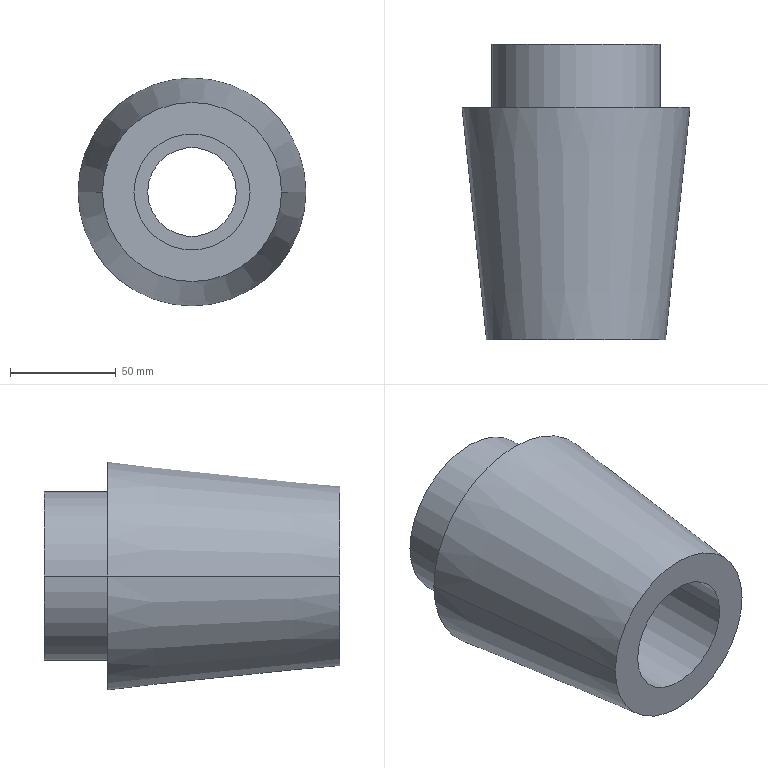Part | STEP file | zhouxin | 1 solid | 18 faces | box 108 x 140 x 108 mm | volume 645082 mm3 | cylinder 10 | plane 6 | cone 2 | commonest cylinder face diameters 4 x4 42 x2 55 x2 80 x2
STEP:
#1=CARTESIAN_POINT('',(2.,-13.333,-32.5));
#2=VERTEX_POINT('',#1);
#3=CARTESIAN_POINT('',(-2.,-13.333,-32.5));
#4=VERTEX_POINT('',#3);
#5=CARTESIAN_POINT('',(0.,-13.333,-32.5));
#6=DIRECTION('',(0.,1.,0.));
#7=DIRECTION('',(-1.,0.,0.));
#8=AXIS2_PLACEMENT_3D('',#5,#6,#7);
#9=CIRCLE('',#8,2.);
#10=EDGE_CURVE('',#2,#4,#9,.T.);
#11=ORIENTED_EDGE('',*,*,#10,.F.);
#12=CARTESIAN_POINT('',(2.,-3.333,-32.5));
#13=VERTEX_POINT('',#12);
#14=CARTESIAN_POINT('',(2.,-13.333,-32.5));
#15=DIRECTION('',(0.,1.,0.));
#16=VECTOR('',#15,1000.);
#17=LINE('',#14,#16);
#18=EDGE_CURVE('',#2,#13,#17,.T.);
#19=ORIENTED_EDGE('',*,*,#18,.T.);
#20=CARTESIAN_POINT('',(-2.,-3.333,-32.5));
#21=VERTEX_POINT('',#20);
#22=CARTESIAN_POINT('',(0.,-3.333,-32.5));
#23=DIRECTION('',(0.,1.,0.));
#24=DIRECTION('',(-1.,0.,0.));
#25=AXIS2_PLACEMENT_3D('',#22,#23,#24);
#26=CIRCLE('',#25,2.);
#27=EDGE_CURVE('',#13,#21,#26,.T.);
#28=ORIENTED_EDGE('',*,*,#27,.T.);
#29=CARTESIAN_POINT('',(-2.,-13.333,-32.5));
#30=DIRECTION('',(0.,1.,0.));
#31=VECTOR('',#30,1000.);
#32=LINE('',#29,#31);
#33=EDGE_CURVE('',#4,#21,#32,.T.);
#34=ORIENTED_EDGE('',*,*,#33,.F.);
#35=EDGE_LOOP('',(#11,#19,#28,#34));
#36=FACE_OUTER_BOUND('',#35,.T.);
#37=CARTESIAN_POINT('',(0.,-13.333,-32.5));
#38=DIRECTION('',(0.,1.,0.));
#39=DIRECTION('',(-1.,0.,0.));
#40=AXIS2_PLACEMENT_3D('',#37,#38,#39);
#41=CYLINDRICAL_SURFACE('',#40,2.);
#42=ADVANCED_FACE('',(#36),#41,.F.);
#43=CARTESIAN_POINT('',(2.,-13.333,32.5));
#44=VERTEX_POINT('',#43);
#45=CARTESIAN_POINT('',(-2.,-13.333,32.5));
#46=VERTEX_POINT('',#45);
#47=CARTESIAN_POINT('',(0.,-13.333,32.5));
#48=DIRECTION('',(0.,1.,0.));
#49=DIRECTION('',(-1.,0.,0.));
#50=AXIS2_PLACEMENT_3D('',#47,#48,#49);
#51=CIRCLE('',#50,2.);
#52=EDGE_CURVE('',#44,#46,#51,.T.);
#53=ORIENTED_EDGE('',*,*,#52,.F.);
#54=CARTESIAN_POINT('',(2.,-3.333,32.5));
#55=VERTEX_POINT('',#54);
#56=CARTESIAN_POINT('',(2.,-13.333,32.5));
#57=DIRECTION('',(0.,1.,0.));
#58=VECTOR('',#57,1000.);
#59=LINE('',#56,#58);
#60=EDGE_CURVE('',#44,#55,#59,.T.);
#61=ORIENTED_EDGE('',*,*,#60,.T.);
#62=CARTESIAN_POINT('',(-2.,-3.333,32.5));
#63=VERTEX_POINT('',#62);
#64=CARTESIAN_POINT('',(0.,-3.333,32.5));
#65=DIRECTION('',(0.,1.,0.));
#66=DIRECTION('',(-1.,0.,0.));
#67=AXIS2_PLACEMENT_3D('',#64,#65,#66);
#68=CIRCLE('',#67,2.);
#69=EDGE_CURVE('',#55,#63,#68,.T.);
#70=ORIENTED_EDGE('',*,*,#69,.T.);
#71=CARTESIAN_POINT('',(-2.,-13.333,32.5));
#72=DIRECTION('',(0.,1.,0.));
#73=VECTOR('',#72,1000.);
#74=LINE('',#71,#73);
#75=EDGE_CURVE('',#46,#63,#74,.T.);
#76=ORIENTED_EDGE('',*,*,#75,.F.);
#77=EDGE_LOOP('',(#53,#61,#70,#76));
#78=FACE_OUTER_BOUND('',#77,.T.);
#79=CARTESIAN_POINT('',(0.,-13.333,32.5));
#80=DIRECTION('',(0.,1.,0.));
#81=DIRECTION('',(-1.,0.,0.));
#82=AXIS2_PLACEMENT_3D('',#79,#80,#81);
#83=CYLINDRICAL_SURFACE('',#82,2.);
#84=ADVANCED_FACE('',(#78),#83,.F.);
#85=CARTESIAN_POINT('',(27.5,-143.333,0.));
#86=VERTEX_POINT('',#85);
#87=CARTESIAN_POINT('',(-27.5,-143.333,0.));
#88=VERTEX_POINT('',#87);
#89=CARTESIAN_POINT('',(0.,-143.333,0.));
#90=DIRECTION('',(0.,1.,0.));
#91=DIRECTION('',(-1.,0.,0.));
#92=AXIS2_PLACEMENT_3D('',#89,#90,#91);
#93=CIRCLE('',#92,27.5);
#94=EDGE_CURVE('',#86,#88,#93,.T.);
#95=ORIENTED_EDGE('',*,*,#94,.F.);
#96=CARTESIAN_POINT('',(27.5,-23.333,0.));
#97=VERTEX_POINT('',#96);
#98=CARTESIAN_POINT('',(27.5,-143.333,0.));
#99=DIRECTION('',(0.,1.,0.));
#100=VECTOR('',#99,1000.);
#101=LINE('',#98,#100);
#102=EDGE_CURVE('',#86,#97,#101,.T.);
#103=ORIENTED_EDGE('',*,*,#102,.T.);
#104=CARTESIAN_POINT('',(-27.5,-23.333,0.));
#105=VERTEX_POINT('',#104);
#106=CARTESIAN_POINT('',(0.,-23.333,0.));
#107=DIRECTION('',(0.,1.,0.));
#108=DIRECTION('',(-1.,0.,0.));
#109=AXIS2_PLACEMENT_3D('',#106,#107,#108);
#110=CIRCLE('',#109,27.5);
#111=EDGE_CURVE('',#97,#105,#110,.T.);
#112=ORIENTED_EDGE('',*,*,#111,.T.);
#113=CARTESIAN_POINT('',(-27.5,-143.333,0.));
#114=DIRECTION('',(0.,1.,0.));
#115=VECTOR('',#114,1000.);
#116=LINE('',#113,#115);
#117=EDGE_CURVE('',#88,#105,#116,.T.);
#118=ORIENTED_EDGE('',*,*,#117,.F.);
#119=EDGE_LOOP('',(#95,#103,#112,#118));
#120=FACE_OUTER_BOUND('',#119,.T.);
#121=CARTESIAN_POINT('',(0.,-143.333,0.));
#122=DIRECTION('',(0.,1.,0.));
#123=DIRECTION('',(-1.,0.,0.));
#124=AXIS2_PLACEMENT_3D('',#121,#122,#123);
#125=CYLINDRICAL_SURFACE('',#124,27.5);
#126=ADVANCED_FACE('',(#120),#125,.F.);
#127=CARTESIAN_POINT('',(21.,-23.333,0.));
#128=VERTEX_POINT('',#127);
#129=CARTESIAN_POINT('',(-21.,-23.333,0.));
#130=VERTEX_POINT('',#129);
#131=CARTESIAN_POINT('',(0.,-23.333,0.));
#132=DIRECTION('',(0.,1.,0.));
#133=DIRECTION('',(-1.,0.,0.));
#134=AXIS2_PLACEMENT_3D('',#131,#132,#133);
#135=CIRCLE('',#134,21.);
#136=EDGE_CURVE('',#128,#130,#135,.T.);
#137=ORIENTED_EDGE('',*,*,#136,.F.);
#138=CARTESIAN_POINT('',(21.,-3.333,0.));
#139=VERTEX_POINT('',#138);
#140=CARTESIAN_POINT('',(21.,-23.333,0.));
#141=DIRECTION('',(0.,1.,0.));
#142=VECTOR('',#141,1000.);
#143=LINE('',#140,#142);
#144=EDGE_CURVE('',#128,#139,#143,.T.);
#145=ORIENTED_EDGE('',*,*,#144,.T.);
#146=CARTESIAN_POINT('',(-21.,-3.333,0.));
#147=VERTEX_POINT('',#146);
#148=CARTESIAN_POINT('',(0.,-3.333,0.));
#149=DIRECTION('',(0.,1.,0.));
#150=DIRECTION('',(-1.,0.,0.));
#151=AXIS2_PLACEMENT_3D('',#148,#149,#150);
#152=CIRCLE('',#151,21.);
#153=EDGE_CURVE('',#139,#147,#152,.T.);
#154=ORIENTED_EDGE('',*,*,#153,.T.);
#155=CARTESIAN_POINT('',(-21.,-23.333,0.));
#156=DIRECTION('',(0.,1.,0.));
#157=VECTOR('',#156,1000.);
#158=LINE('',#155,#157);
#159=EDGE_CURVE('',#130,#147,#158,.T.);
#160=ORIENTED_EDGE('',*,*,#159,.F.);
#161=EDGE_LOOP('',(#137,#145,#154,#160));
#162=FACE_OUTER_BOUND('',#161,.T.);
#163=CARTESIAN_POINT('',(0.,-23.333,0.));
#164=DIRECTION('',(0.,1.,0.));
#165=DIRECTION('',(-1.,0.,0.));
#166=AXIS2_PLACEMENT_3D('',#163,#164,#165);
#167=CYLINDRICAL_SURFACE('',#166,21.);
#168=ADVANCED_FACE('',(#162),#167,.F.);
#169=CARTESIAN_POINT('',(-42.439,-143.333,0.));
#170=VERTEX_POINT('',#169);
#171=CARTESIAN_POINT('',(42.439,-143.333,0.));
#172=VERTEX_POINT('',#171);
#173=CARTESIAN_POINT('',(0.,-143.333,0.));
#174=DIRECTION('',(0.,1.,0.));
#175=DIRECTION('',(-1.,0.,0.));
#176=AXIS2_PLACEMENT_3D('',#173,#174,#175);
#177=CIRCLE('',#176,42.439);
#178=EDGE_CURVE('',#170,#172,#177,.T.);
#179=ORIENTED_EDGE('',*,*,#178,.T.);
#180=CARTESIAN_POINT('',(54.,-33.333,0.));
#181=VERTEX_POINT('',#180);
#182=CARTESIAN_POINT('',(42.439,-143.333,0.));
#183=DIRECTION('',(0.1045,0.9945,0.));
#184=VECTOR('',#183,1000.);
#185=LINE('',#182,#184);
#186=EDGE_CURVE('',#172,#181,#185,.T.);
#187=ORIENTED_EDGE('',*,*,#186,.T.);
#188=CARTESIAN_POINT('',(-54.,-33.333,0.));
#189=VERTEX_POINT('',#188);
#190=CARTESIAN_POINT('',(0.,-33.333,0.));
#191=DIRECTION('',(0.,1.,0.));
#192=DIRECTION('',(-1.,0.,0.));
#193=AXIS2_PLACEMENT_3D('',#190,#191,#192);
#194=CIRCLE('',#193,54.);
#195=EDGE_CURVE('',#189,#181,#194,.T.);
#196=ORIENTED_EDGE('',*,*,#195,.F.);
#197=CARTESIAN_POINT('',(-42.439,-143.333,0.));
#198=DIRECTION('',(-0.1045,0.9945,0.));
#199=VECTOR('',#198,1000.);
#200=LINE('',#197,#199);
#201=EDGE_CURVE('',#170,#189,#200,.T.);
#202=ORIENTED_EDGE('',*,*,#201,.F.);
#203=EDGE_LOOP('',(#179,#187,#196,#202));
#204=FACE_OUTER_BOUND('',#203,.T.);
#205=CARTESIAN_POINT('',(0.,-143.333,0.));
#206=DIRECTION('',(0.,1.,0.));
#207=DIRECTION('',(-1.,0.,0.));
#208=AXIS2_PLACEMENT_3D('',#205,#206,#207);
#209=CONICAL_SURFACE('',#208,42.439,0.1047);
#210=ADVANCED_FACE('',(#204),#209,.T.);
#211=CARTESIAN_POINT('',(-40.,-33.333,0.));
#212=VERTEX_POINT('',#211);
#213=CARTESIAN_POINT('',(40.,-33.333,0.));
#214=VERTEX_POINT('',#213);
#215=CARTESIAN_POINT('',(0.,-33.333,0.));
#216=DIRECTION('',(0.,1.,0.));
#217=DIRECTION('',(-1.,0.,0.));
#218=AXIS2_PLACEMENT_3D('',#215,#216,#217);
#219=CIRCLE('',#218,40.);
#220=EDGE_CURVE('',#212,#214,#219,.T.);
#221=ORIENTED_EDGE('',*,*,#220,.T.);
#222=CARTESIAN_POINT('',(40.,-3.333,0.));
#223=VERTEX_POINT('',#222);
#224=CARTESIAN_POINT('',(40.,-3.333,0.));
#225=DIRECTION('',(0.,1.,0.));
#226=VECTOR('',#225,1000.);
#227=LINE('',#224,#226);
#228=EDGE_CURVE('',#214,#223,#227,.T.);
#229=ORIENTED_EDGE('',*,*,#228,.T.);
#230=CARTESIAN_POINT('',(-40.,-3.333,0.));
#231=VERTEX_POINT('',#230);
#232=CARTESIAN_POINT('',(0.,-3.333,0.));
#233=DIRECTION('',(0.,1.,0.));
#234=DIRECTION('',(-1.,0.,0.));
#235=AXIS2_PLACEMENT_3D('',#232,#233,#234);
#236=CIRCLE('',#235,40.);
#237=EDGE_CURVE('',#231,#223,#236,.T.);
#238=ORIENTED_EDGE('',*,*,#237,.F.);
#239=CARTESIAN_POINT('',(-40.,-3.333,0.));
#240=DIRECTION('',(0.,1.,0.));
#241=VECTOR('',#240,1000.);
#242=LINE('',#239,#241);
#243=EDGE_CURVE('',#212,#231,#242,.T.);
#244=ORIENTED_EDGE('',*,*,#243,.F.);
#245=EDGE_LOOP('',(#221,#229,#238,#244));
#246=FACE_OUTER_BOUND('',#245,.T.);
#247=CARTESIAN_POINT('',(0.,-3.333,0.));
#248=DIRECTION('',(0.,1.,0.));
#249=DIRECTION('',(-1.,0.,0.));
#250=AXIS2_PLACEMENT_3D('',#247,#248,#249);
#251=CYLINDRICAL_SURFACE('',#250,40.);
#252=ADVANCED_FACE('',(#246),#251,.T.);
#253=CARTESIAN_POINT('',(0.,-3.333,-32.5));
#254=DIRECTION('',(0.,1.,0.));
#255=DIRECTION('',(-1.,0.,0.));
#256=AXIS2_PLACEMENT_3D('',#253,#254,#255);
#257=CIRCLE('',#256,2.);
#258=EDGE_CURVE('',#21,#13,#257,.T.);
#259=ORIENTED_EDGE('',*,*,#258,.F.);
#260=ORIENTED_EDGE('',*,*,#27,.F.);
#261=EDGE_LOOP('',(#259,#260));
#262=FACE_BOUND('',#261,.T.);
#263=CARTESIAN_POINT('',(0.,-3.333,32.5));
#264=DIRECTION('',(0.,1.,0.));
#265=DIRECTION('',(-1.,0.,0.));
#266=AXIS2_PLACEMENT_3D('',#263,#264,#265);
#267=CIRCLE('',#266,2.);
#268=EDGE_CURVE('',#63,#55,#267,.T.);
#269=ORIENTED_EDGE('',*,*,#268,.F.);
#270=ORIENTED_EDGE('',*,*,#69,.F.);
#271=EDGE_LOOP('',(#269,#270));
#272=FACE_BOUND('',#271,.T.);
#273=CARTESIAN_POINT('',(0.,-3.333,0.));
#274=DIRECTION('',(0.,1.,0.));
#275=DIRECTION('',(-1.,0.,0.));
#276=AXIS2_PLACEMENT_3D('',#273,#274,#275);
#277=CIRCLE('',#276,21.);
#278=EDGE_CURVE('',#147,#139,#277,.T.);
#279=ORIENTED_EDGE('',*,*,#278,.F.);
#280=ORIENTED_EDGE('',*,*,#153,.F.);
#281=EDGE_LOOP('',(#279,#280));
#282=FACE_BOUND('',#281,.T.);
#283=ORIENTED_EDGE('',*,*,#237,.T.);
#284=CARTESIAN_POINT('',(0.,-3.333,0.));
#285=DIRECTION('',(0.,1.,0.));
#286=DIRECTION('',(-1.,0.,0.));
#287=AXIS2_PLACEMENT_3D('',#284,#285,#286);
#288=CIRCLE('',#287,40.);
#289=EDGE_CURVE('',#223,#231,#288,.T.);
#290=ORIENTED_EDGE('',*,*,#289,.T.);
#291=EDGE_LOOP('',(#283,#290));
#292=FACE_OUTER_BOUND('',#291,.T.);
#293=CARTESIAN_POINT('',(0.,-3.333,0.));
#294=DIRECTION('',(0.,-1.,0.));
#295=DIRECTION('',(1.,0.,0.));
#296=AXIS2_PLACEMENT_3D('',#293,#294,#295);
#297=PLANE('',#296);
#298=ADVANCED_FACE('',(#262,#272,#282,#292),#297,.F.);
#299=ORIENTED_EDGE('',*,*,#228,.F.);
#300=CARTESIAN_POINT('',(0.,-33.333,0.));
#301=DIRECTION('',(0.,1.,0.));
#302=DIRECTION('',(-1.,0.,0.));
#303=AXIS2_PLACEMENT_3D('',#300,#301,#302);
#304=CIRCLE('',#303,40.);
#305=EDGE_CURVE('',#214,#212,#304,.T.);
#306=ORIENTED_EDGE('',*,*,#305,.T.);
#307=ORIENTED_EDGE('',*,*,#243,.T.);
#308=ORIENTED_EDGE('',*,*,#289,.F.);
#309=EDGE_LOOP('',(#299,#306,#307,#308));
#310=FACE_OUTER_BOUND('',#309,.T.);
#311=CARTESIAN_POINT('',(0.,-3.333,0.));
#312=DIRECTION('',(0.,1.,0.));
#313=DIRECTION('',(-1.,0.,0.));
#314=AXIS2_PLACEMENT_3D('',#311,#312,#313);
#315=CYLINDRICAL_SURFACE('',#314,40.);
#316=ADVANCED_FACE('',(#310),#315,.T.);
#317=ORIENTED_EDGE('',*,*,#220,.F.);
#318=ORIENTED_EDGE('',*,*,#305,.F.);
#319=EDGE_LOOP('',(#317,#318));
#320=FACE_BOUND('',#319,.T.);
#321=ORIENTED_EDGE('',*,*,#195,.T.);
#322=CARTESIAN_POINT('',(0.,-33.333,0.));
#323=DIRECTION('',(0.,1.,0.));
#324=DIRECTION('',(-1.,0.,0.));
#325=AXIS2_PLACEMENT_3D('',#322,#323,#324);
#326=CIRCLE('',#325,54.);
#327=EDGE_CURVE('',#181,#189,#326,.T.);
#328=ORIENTED_EDGE('',*,*,#327,.T.);
#329=EDGE_LOOP('',(#321,#328));
#330=FACE_OUTER_BOUND('',#329,.T.);
#331=CARTESIAN_POINT('',(40.,-33.333,0.));
#332=DIRECTION('',(0.,-1.,0.));
#333=DIRECTION('',(1.,0.,0.));
#334=AXIS2_PLACEMENT_3D('',#331,#332,#333);
#335=PLANE('',#334);
#336=ADVANCED_FACE('',(#320,#330),#335,.F.);
#337=ORIENTED_EDGE('',*,*,#186,.F.);
#338=CARTESIAN_POINT('',(0.,-143.333,0.));
#339=DIRECTION('',(0.,1.,0.));
#340=DIRECTION('',(-1.,0.,0.));
#341=AXIS2_PLACEMENT_3D('',#338,#339,#340);
#342=CIRCLE('',#341,42.439);
#343=EDGE_CURVE('',#172,#170,#342,.T.);
#344=ORIENTED_EDGE('',*,*,#343,.T.);
#345=ORIENTED_EDGE('',*,*,#201,.T.);
#346=ORIENTED_EDGE('',*,*,#327,.F.);
#347=EDGE_LOOP('',(#337,#344,#345,#346));
#348=FACE_OUTER_BOUND('',#347,.T.);
#349=CARTESIAN_POINT('',(0.,-143.333,0.));
#350=DIRECTION('',(0.,1.,0.));
#351=DIRECTION('',(-1.,0.,0.));
#352=AXIS2_PLACEMENT_3D('',#349,#350,#351);
#353=CONICAL_SURFACE('',#352,42.439,0.1047);
#354=ADVANCED_FACE('',(#348),#353,.T.);
#355=CARTESIAN_POINT('',(0.,-143.333,0.));
#356=DIRECTION('',(0.,1.,0.));
#357=DIRECTION('',(-1.,0.,0.));
#358=AXIS2_PLACEMENT_3D('',#355,#356,#357);
#359=CIRCLE('',#358,27.5);
#360=EDGE_CURVE('',#88,#86,#359,.T.);
#361=ORIENTED_EDGE('',*,*,#360,.T.);
#362=ORIENTED_EDGE('',*,*,#94,.T.);
#363=EDGE_LOOP('',(#361,#362));
#364=FACE_BOUND('',#363,.T.);
#365=ORIENTED_EDGE('',*,*,#178,.F.);
#366=ORIENTED_EDGE('',*,*,#343,.F.);
#367=EDGE_LOOP('',(#365,#366));
#368=FACE_OUTER_BOUND('',#367,.T.);
#369=CARTESIAN_POINT('',(42.439,-143.333,0.));
#370=DIRECTION('',(0.,1.,0.));
#371=DIRECTION('',(-1.,0.,0.));
#372=AXIS2_PLACEMENT_3D('',#369,#370,#371);
#373=PLANE('',#372);
#374=ADVANCED_FACE('',(#364,#368),#373,.F.);
#375=ORIENTED_EDGE('',*,*,#144,.F.);
#376=CARTESIAN_POINT('',(0.,-23.333,0.));
#377=DIRECTION('',(0.,1.,0.));
#378=DIRECTION('',(-1.,0.,0.));
#379=AXIS2_PLACEMENT_3D('',#376,#377,#378);
#380=CIRCLE('',#379,21.);
#381=EDGE_CURVE('',#130,#128,#380,.T.);
#382=ORIENTED_EDGE('',*,*,#381,.F.);
#383=ORIENTED_EDGE('',*,*,#159,.T.);
#384=ORIENTED_EDGE('',*,*,#278,.T.);
#385=EDGE_LOOP('',(#375,#382,#383,#384));
#386=FACE_OUTER_BOUND('',#385,.T.);
#387=CARTESIAN_POINT('',(0.,-23.333,0.));
#388=DIRECTION('',(0.,1.,0.));
#389=DIRECTION('',(-1.,0.,0.));
#390=AXIS2_PLACEMENT_3D('',#387,#388,#389);
#391=CYLINDRICAL_SURFACE('',#390,21.);
#392=ADVANCED_FACE('',(#386),#391,.F.);
#393=ORIENTED_EDGE('',*,*,#102,.F.);
#394=ORIENTED_EDGE('',*,*,#360,.F.);
#395=ORIENTED_EDGE('',*,*,#117,.T.);
#396=CARTESIAN_POINT('',(0.,-23.333,0.));
#397=DIRECTION('',(0.,1.,0.));
#398=DIRECTION('',(-1.,0.,0.));
#399=AXIS2_PLACEMENT_3D('',#396,#397,#398);
#400=CIRCLE('',#399,27.5);
#401=EDGE_CURVE('',#105,#97,#400,.T.);
#402=ORIENTED_EDGE('',*,*,#401,.T.);
#403=EDGE_LOOP('',(#393,#394,#395,#402));
#404=FACE_OUTER_BOUND('',#403,.T.);
#405=CARTESIAN_POINT('',(0.,-143.333,0.));
#406=DIRECTION('',(0.,1.,0.));
#407=DIRECTION('',(-1.,0.,0.));
#408=AXIS2_PLACEMENT_3D('',#405,#406,#407);
#409=CYLINDRICAL_SURFACE('',#408,27.5);
#410=ADVANCED_FACE('',(#404),#409,.F.);
#411=ORIENTED_EDGE('',*,*,#381,.T.);
#412=ORIENTED_EDGE('',*,*,#136,.T.);
#413=EDGE_LOOP('',(#411,#412));
#414=FACE_BOUND('',#413,.T.);
#415=ORIENTED_EDGE('',*,*,#401,.F.);
#416=ORIENTED_EDGE('',*,*,#111,.F.);
#417=EDGE_LOOP('',(#415,#416));
#418=FACE_OUTER_BOUND('',#417,.T.);
#419=CARTESIAN_POINT('',(0.,-23.333,0.));
#420=DIRECTION('',(0.,1.,0.));
#421=DIRECTION('',(-1.,0.,0.));
#422=AXIS2_PLACEMENT_3D('',#419,#420,#421);
#423=PLANE('',#422);
#424=ADVANCED_FACE('',(#414,#418),#423,.F.);
#425=ORIENTED_EDGE('',*,*,#60,.F.);
#426=CARTESIAN_POINT('',(0.,-13.333,32.5));
#427=DIRECTION('',(0.,1.,0.));
#428=DIRECTION('',(-1.,0.,0.));
#429=AXIS2_PLACEMENT_3D('',#426,#427,#428);
#430=CIRCLE('',#429,2.);
#431=EDGE_CURVE('',#46,#44,#430,.T.);
#432=ORIENTED_EDGE('',*,*,#431,.F.);
#433=ORIENTED_EDGE('',*,*,#75,.T.);
#434=ORIENTED_EDGE('',*,*,#268,.T.);
#435=EDGE_LOOP('',(#425,#432,#433,#434));
#436=FACE_OUTER_BOUND('',#435,.T.);
#437=CARTESIAN_POINT('',(0.,-13.333,32.5));
#438=DIRECTION('',(0.,1.,0.));
#439=DIRECTION('',(-1.,0.,0.));
#440=AXIS2_PLACEMENT_3D('',#437,#438,#439);
#441=CYLINDRICAL_SURFACE('',#440,2.);
#442=ADVANCED_FACE('',(#436),#441,.F.);
#443=ORIENTED_EDGE('',*,*,#431,.T.);
#444=ORIENTED_EDGE('',*,*,#52,.T.);
#445=EDGE_LOOP('',(#443,#444));
#446=FACE_OUTER_BOUND('',#445,.T.);
#447=CARTESIAN_POINT('',(0.,-13.333,32.5));
#448=DIRECTION('',(0.,1.,0.));
#449=DIRECTION('',(-1.,0.,0.));
#450=AXIS2_PLACEMENT_3D('',#447,#448,#449);
#451=PLANE('',#450);
#452=ADVANCED_FACE('',(#446),#451,.T.);
#453=ORIENTED_EDGE('',*,*,#18,.F.);
#454=CARTESIAN_POINT('',(0.,-13.333,-32.5));
#455=DIRECTION('',(0.,1.,0.));
#456=DIRECTION('',(-1.,0.,0.));
#457=AXIS2_PLACEMENT_3D('',#454,#455,#456);
#458=CIRCLE('',#457,2.);
#459=EDGE_CURVE('',#4,#2,#458,.T.);
#460=ORIENTED_EDGE('',*,*,#459,.F.);
#461=ORIENTED_EDGE('',*,*,#33,.T.);
#462=ORIENTED_EDGE('',*,*,#258,.T.);
#463=EDGE_LOOP('',(#453,#460,#461,#462));
#464=FACE_OUTER_BOUND('',#463,.T.);
#465=CARTESIAN_POINT('',(0.,-13.333,-32.5));
#466=DIRECTION('',(0.,1.,0.));
#467=DIRECTION('',(-1.,0.,0.));
#468=AXIS2_PLACEMENT_3D('',#465,#466,#467);
#469=CYLINDRICAL_SURFACE('',#468,2.);
#470=ADVANCED_FACE('',(#464),#469,.F.);
#471=ORIENTED_EDGE('',*,*,#459,.T.);
#472=ORIENTED_EDGE('',*,*,#10,.T.);
#473=EDGE_LOOP('',(#471,#472));
#474=FACE_OUTER_BOUND('',#473,.T.);
#475=CARTESIAN_POINT('',(0.,-13.333,-32.5));
#476=DIRECTION('',(0.,1.,0.));
#477=DIRECTION('',(-1.,0.,0.));
#478=AXIS2_PLACEMENT_3D('',#475,#476,#477);
#479=PLANE('',#478);
#480=ADVANCED_FACE('',(#474),#479,.T.);
#481=CLOSED_SHELL('',(#42,#84,#126,#168,#210,#252,#298,#316,#336,#354,#374,#392,#410,#424,#442,#452,#470,#480));
#482=MANIFOLD_SOLID_BREP('',#481);
#483=CARTESIAN_POINT('',(0.,0.,0.));
#484=DIRECTION('',(0.,0.,1.));
#485=DIRECTION('',(1.,0.,0.));
#486=AXIS2_PLACEMENT_3D('',#483,#484,#485);
#487=(LENGTH_UNIT()NAMED_UNIT(*)SI_UNIT(.MILLI.,.METRE.));
#488=UNCERTAINTY_MEASURE_WITH_UNIT(LENGTH_MEASURE(0.00001),#487,'','');
#489=(NAMED_UNIT(*)PLANE_ANGLE_UNIT()SI_UNIT($,.RADIAN.));
#490=(NAMED_UNIT(*)SI_UNIT($,.STERADIAN.)SOLID_ANGLE_UNIT());
#491=(GEOMETRIC_REPRESENTATION_CONTEXT(3)GLOBAL_UNCERTAINTY_ASSIGNED_CONTEXT((#488))GLOBAL_UNIT_ASSIGNED_CONTEXT((#487,#489,#490))REPRESENTATION_CONTEXT('',''));
#492=ADVANCED_BREP_SHAPE_REPRESENTATION('',(#482,#486),#491);